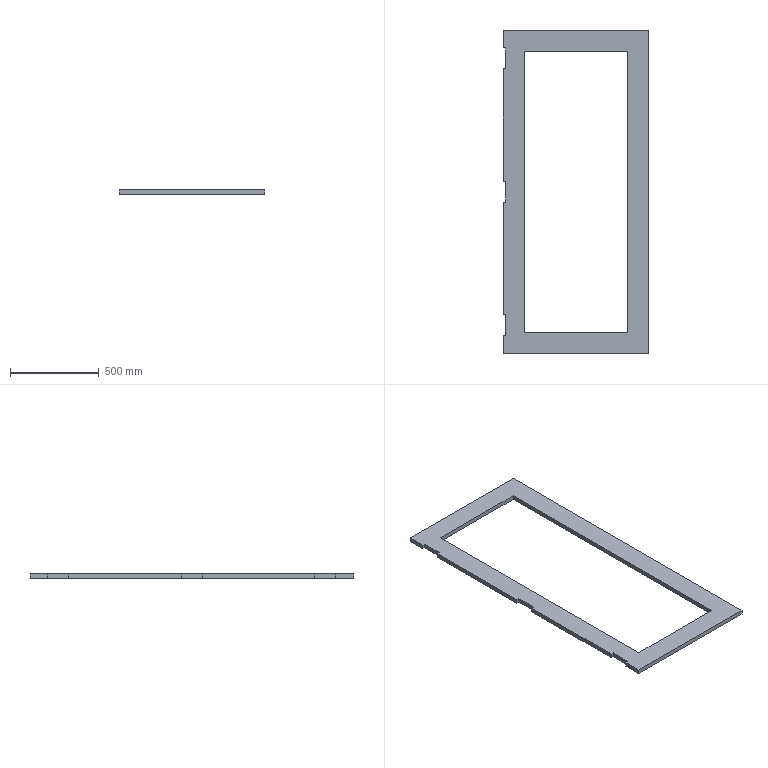Part | SolidWorks | features ICE 2, Extrusion 1 | 1 solid | 22 faces | box 820 x 1820 x 25 mm | volume 14268375 mm3 | plane 22
STEP:
#1=CARTESIAN_POINT('',(-410.,693.,0.));
#2=VERTEX_POINT('',#1);
#3=CARTESIAN_POINT('',(-410.,60.,0.));
#4=VERTEX_POINT('',#3);
#5=CARTESIAN_POINT('',(-410.,910.,0.));
#6=DIRECTION('',(0.,-1.,0.));
#7=VECTOR('',#6,1000.);
#8=LINE('',#5,#7);
#9=EDGE_CURVE('',#2,#4,#8,.T.);
#10=ORIENTED_EDGE('',*,*,#9,.T.);
#11=CARTESIAN_POINT('',(-410.,60.,25.));
#12=VERTEX_POINT('',#11);
#13=CARTESIAN_POINT('',(-410.,60.,0.));
#14=DIRECTION('',(0.,0.,1.));
#15=VECTOR('',#14,1000.);
#16=LINE('',#13,#15);
#17=EDGE_CURVE('',#4,#12,#16,.T.);
#18=ORIENTED_EDGE('',*,*,#17,.T.);
#19=CARTESIAN_POINT('',(-410.,693.,25.));
#20=VERTEX_POINT('',#19);
#21=CARTESIAN_POINT('',(-410.,910.,25.));
#22=DIRECTION('',(0.,-1.,0.));
#23=VECTOR('',#22,1000.);
#24=LINE('',#21,#23);
#25=EDGE_CURVE('',#20,#12,#24,.T.);
#26=ORIENTED_EDGE('',*,*,#25,.F.);
#27=CARTESIAN_POINT('',(-410.,693.,0.));
#28=DIRECTION('',(0.,0.,1.));
#29=VECTOR('',#28,1000.);
#30=LINE('',#27,#29);
#31=EDGE_CURVE('',#2,#20,#30,.T.);
#32=ORIENTED_EDGE('',*,*,#31,.F.);
#33=EDGE_LOOP('',(#10,#18,#26,#32));
#34=FACE_OUTER_BOUND('',#33,.T.);
#35=CARTESIAN_POINT('',(-410.,910.,25.));
#36=DIRECTION('',(1.,0.,0.));
#37=DIRECTION('',(0.,1.,0.));
#38=AXIS2_PLACEMENT_3D('',#35,#36,#37);
#39=PLANE('',#38);
#40=ADVANCED_FACE('',(#34),#39,.F.);
#41=CARTESIAN_POINT('',(-410.,910.,0.));
#42=VERTEX_POINT('',#41);
#43=CARTESIAN_POINT('',(-410.,810.,0.));
#44=VERTEX_POINT('',#43);
#45=CARTESIAN_POINT('',(-410.,910.,0.));
#46=DIRECTION('',(0.,-1.,0.));
#47=VECTOR('',#46,1000.);
#48=LINE('',#45,#47);
#49=EDGE_CURVE('',#42,#44,#48,.T.);
#50=ORIENTED_EDGE('',*,*,#49,.T.);
#51=CARTESIAN_POINT('',(-410.,810.,25.));
#52=VERTEX_POINT('',#51);
#53=CARTESIAN_POINT('',(-410.,810.,0.));
#54=DIRECTION('',(0.,0.,1.));
#55=VECTOR('',#54,1000.);
#56=LINE('',#53,#55);
#57=EDGE_CURVE('',#44,#52,#56,.T.);
#58=ORIENTED_EDGE('',*,*,#57,.T.);
#59=CARTESIAN_POINT('',(-410.,910.,25.));
#60=VERTEX_POINT('',#59);
#61=CARTESIAN_POINT('',(-410.,910.,25.));
#62=DIRECTION('',(0.,-1.,0.));
#63=VECTOR('',#62,1000.);
#64=LINE('',#61,#63);
#65=EDGE_CURVE('',#60,#52,#64,.T.);
#66=ORIENTED_EDGE('',*,*,#65,.F.);
#67=CARTESIAN_POINT('',(-410.,910.,25.));
#68=DIRECTION('',(0.,0.,-1.));
#69=VECTOR('',#68,1000.);
#70=LINE('',#67,#69);
#71=EDGE_CURVE('',#60,#42,#70,.T.);
#72=ORIENTED_EDGE('',*,*,#71,.T.);
#73=EDGE_LOOP('',(#50,#58,#66,#72));
#74=FACE_OUTER_BOUND('',#73,.T.);
#75=CARTESIAN_POINT('',(-410.,910.,25.));
#76=DIRECTION('',(1.,0.,0.));
#77=DIRECTION('',(0.,1.,0.));
#78=AXIS2_PLACEMENT_3D('',#75,#76,#77);
#79=PLANE('',#78);
#80=ADVANCED_FACE('',(#74),#79,.F.);
#81=CARTESIAN_POINT('',(-410.,-57.,25.));
#82=VERTEX_POINT('',#81);
#83=CARTESIAN_POINT('',(-410.,-690.,25.));
#84=VERTEX_POINT('',#83);
#85=CARTESIAN_POINT('',(-410.,910.,25.));
#86=DIRECTION('',(0.,-1.,0.));
#87=VECTOR('',#86,1000.);
#88=LINE('',#85,#87);
#89=EDGE_CURVE('',#82,#84,#88,.T.);
#90=ORIENTED_EDGE('',*,*,#89,.F.);
#91=CARTESIAN_POINT('',(-410.,-57.,0.));
#92=VERTEX_POINT('',#91);
#93=CARTESIAN_POINT('',(-410.,-57.,0.));
#94=DIRECTION('',(0.,0.,1.));
#95=VECTOR('',#94,1000.);
#96=LINE('',#93,#95);
#97=EDGE_CURVE('',#92,#82,#96,.T.);
#98=ORIENTED_EDGE('',*,*,#97,.F.);
#99=CARTESIAN_POINT('',(-410.,-690.,0.));
#100=VERTEX_POINT('',#99);
#101=CARTESIAN_POINT('',(-410.,910.,0.));
#102=DIRECTION('',(0.,-1.,0.));
#103=VECTOR('',#102,1000.);
#104=LINE('',#101,#103);
#105=EDGE_CURVE('',#92,#100,#104,.T.);
#106=ORIENTED_EDGE('',*,*,#105,.T.);
#107=CARTESIAN_POINT('',(-410.,-690.,0.));
#108=DIRECTION('',(0.,0.,1.));
#109=VECTOR('',#108,1000.);
#110=LINE('',#107,#109);
#111=EDGE_CURVE('',#100,#84,#110,.T.);
#112=ORIENTED_EDGE('',*,*,#111,.T.);
#113=EDGE_LOOP('',(#90,#98,#106,#112));
#114=FACE_OUTER_BOUND('',#113,.T.);
#115=CARTESIAN_POINT('',(-410.,910.,25.));
#116=DIRECTION('',(1.,0.,0.));
#117=DIRECTION('',(0.,1.,0.));
#118=AXIS2_PLACEMENT_3D('',#115,#116,#117);
#119=PLANE('',#118);
#120=ADVANCED_FACE('',(#114),#119,.F.);
#121=CARTESIAN_POINT('',(410.,-910.,0.));
#122=VERTEX_POINT('',#121);
#123=CARTESIAN_POINT('',(410.,910.,0.));
#124=VERTEX_POINT('',#123);
#125=CARTESIAN_POINT('',(410.,910.,0.));
#126=DIRECTION('',(0.,1.,0.));
#127=VECTOR('',#126,1000.);
#128=LINE('',#125,#127);
#129=EDGE_CURVE('',#122,#124,#128,.T.);
#130=ORIENTED_EDGE('',*,*,#129,.T.);
#131=CARTESIAN_POINT('',(410.,910.,25.));
#132=VERTEX_POINT('',#131);
#133=CARTESIAN_POINT('',(410.,910.,25.));
#134=DIRECTION('',(0.,0.,-1.));
#135=VECTOR('',#134,1000.);
#136=LINE('',#133,#135);
#137=EDGE_CURVE('',#132,#124,#136,.T.);
#138=ORIENTED_EDGE('',*,*,#137,.F.);
#139=CARTESIAN_POINT('',(410.,-910.,25.));
#140=VERTEX_POINT('',#139);
#141=CARTESIAN_POINT('',(410.,910.,25.));
#142=DIRECTION('',(0.,1.,0.));
#143=VECTOR('',#142,1000.);
#144=LINE('',#141,#143);
#145=EDGE_CURVE('',#140,#132,#144,.T.);
#146=ORIENTED_EDGE('',*,*,#145,.F.);
#147=CARTESIAN_POINT('',(410.,-910.,25.));
#148=DIRECTION('',(0.,0.,-1.));
#149=VECTOR('',#148,1000.);
#150=LINE('',#147,#149);
#151=EDGE_CURVE('',#140,#122,#150,.T.);
#152=ORIENTED_EDGE('',*,*,#151,.T.);
#153=EDGE_LOOP('',(#130,#138,#146,#152));
#154=FACE_OUTER_BOUND('',#153,.T.);
#155=CARTESIAN_POINT('',(410.,910.,25.));
#156=DIRECTION('',(-1.,0.,0.));
#157=DIRECTION('',(0.,-1.,0.));
#158=AXIS2_PLACEMENT_3D('',#155,#156,#157);
#159=PLANE('',#158);
#160=ADVANCED_FACE('',(#154),#159,.F.);
#161=CARTESIAN_POINT('',(-410.,910.,0.));
#162=DIRECTION('',(-1.,0.,0.));
#163=VECTOR('',#162,1000.);
#164=LINE('',#161,#163);
#165=EDGE_CURVE('',#124,#42,#164,.T.);
#166=ORIENTED_EDGE('',*,*,#165,.T.);
#167=ORIENTED_EDGE('',*,*,#71,.F.);
#168=CARTESIAN_POINT('',(-410.,910.,25.));
#169=DIRECTION('',(-1.,0.,0.));
#170=VECTOR('',#169,1000.);
#171=LINE('',#168,#170);
#172=EDGE_CURVE('',#132,#60,#171,.T.);
#173=ORIENTED_EDGE('',*,*,#172,.F.);
#174=ORIENTED_EDGE('',*,*,#137,.T.);
#175=EDGE_LOOP('',(#166,#167,#173,#174));
#176=FACE_OUTER_BOUND('',#175,.T.);
#177=CARTESIAN_POINT('',(-410.,910.,25.));
#178=DIRECTION('',(0.,-1.,0.));
#179=DIRECTION('',(0.,0.,-1.));
#180=AXIS2_PLACEMENT_3D('',#177,#178,#179);
#181=PLANE('',#180);
#182=ADVANCED_FACE('',(#176),#181,.F.);
#183=CARTESIAN_POINT('',(-410.,-807.,25.));
#184=VERTEX_POINT('',#183);
#185=CARTESIAN_POINT('',(-410.,-910.,25.));
#186=VERTEX_POINT('',#185);
#187=CARTESIAN_POINT('',(-410.,910.,25.));
#188=DIRECTION('',(0.,-1.,0.));
#189=VECTOR('',#188,1000.);
#190=LINE('',#187,#189);
#191=EDGE_CURVE('',#184,#186,#190,.T.);
#192=ORIENTED_EDGE('',*,*,#191,.F.);
#193=CARTESIAN_POINT('',(-410.,-807.,0.));
#194=VERTEX_POINT('',#193);
#195=CARTESIAN_POINT('',(-410.,-807.,0.));
#196=DIRECTION('',(0.,0.,1.));
#197=VECTOR('',#196,1000.);
#198=LINE('',#195,#197);
#199=EDGE_CURVE('',#194,#184,#198,.T.);
#200=ORIENTED_EDGE('',*,*,#199,.F.);
#201=CARTESIAN_POINT('',(-410.,-910.,0.));
#202=VERTEX_POINT('',#201);
#203=CARTESIAN_POINT('',(-410.,910.,0.));
#204=DIRECTION('',(0.,-1.,0.));
#205=VECTOR('',#204,1000.);
#206=LINE('',#203,#205);
#207=EDGE_CURVE('',#194,#202,#206,.T.);
#208=ORIENTED_EDGE('',*,*,#207,.T.);
#209=CARTESIAN_POINT('',(-410.,-910.,25.));
#210=DIRECTION('',(0.,0.,-1.));
#211=VECTOR('',#210,1000.);
#212=LINE('',#209,#211);
#213=EDGE_CURVE('',#186,#202,#212,.T.);
#214=ORIENTED_EDGE('',*,*,#213,.F.);
#215=EDGE_LOOP('',(#192,#200,#208,#214));
#216=FACE_OUTER_BOUND('',#215,.T.);
#217=CARTESIAN_POINT('',(-410.,910.,25.));
#218=DIRECTION('',(1.,0.,0.));
#219=DIRECTION('',(0.,1.,0.));
#220=AXIS2_PLACEMENT_3D('',#217,#218,#219);
#221=PLANE('',#220);
#222=ADVANCED_FACE('',(#216),#221,.F.);
#223=CARTESIAN_POINT('',(-410.,-910.,0.));
#224=DIRECTION('',(1.,0.,0.));
#225=VECTOR('',#224,1000.);
#226=LINE('',#223,#225);
#227=EDGE_CURVE('',#202,#122,#226,.T.);
#228=ORIENTED_EDGE('',*,*,#227,.T.);
#229=ORIENTED_EDGE('',*,*,#151,.F.);
#230=CARTESIAN_POINT('',(-410.,-910.,25.));
#231=DIRECTION('',(1.,0.,0.));
#232=VECTOR('',#231,1000.);
#233=LINE('',#230,#232);
#234=EDGE_CURVE('',#186,#140,#233,.T.);
#235=ORIENTED_EDGE('',*,*,#234,.F.);
#236=ORIENTED_EDGE('',*,*,#213,.T.);
#237=EDGE_LOOP('',(#228,#229,#235,#236));
#238=FACE_OUTER_BOUND('',#237,.T.);
#239=CARTESIAN_POINT('',(-410.,-910.,25.));
#240=DIRECTION('',(0.,1.,0.));
#241=DIRECTION('',(0.,0.,1.));
#242=AXIS2_PLACEMENT_3D('',#239,#240,#241);
#243=PLANE('',#242);
#244=ADVANCED_FACE('',(#238),#243,.F.);
#245=CARTESIAN_POINT('',(-395.,60.,25.));
#246=VERTEX_POINT('',#245);
#247=CARTESIAN_POINT('',(-410.,60.,25.));
#248=DIRECTION('',(-1.,0.,0.));
#249=VECTOR('',#248,1000.);
#250=LINE('',#247,#249);
#251=EDGE_CURVE('',#246,#12,#250,.T.);
#252=ORIENTED_EDGE('',*,*,#251,.F.);
#253=CARTESIAN_POINT('',(-395.,-57.,25.));
#254=VERTEX_POINT('',#253);
#255=CARTESIAN_POINT('',(-395.,60.,25.));
#256=DIRECTION('',(0.,1.,0.));
#257=VECTOR('',#256,1000.);
#258=LINE('',#255,#257);
#259=EDGE_CURVE('',#254,#246,#258,.T.);
#260=ORIENTED_EDGE('',*,*,#259,.F.);
#261=CARTESIAN_POINT('',(-410.,-57.,25.));
#262=DIRECTION('',(1.,0.,0.));
#263=VECTOR('',#262,1000.);
#264=LINE('',#261,#263);
#265=EDGE_CURVE('',#82,#254,#264,.T.);
#266=ORIENTED_EDGE('',*,*,#265,.F.);
#267=ORIENTED_EDGE('',*,*,#89,.T.);
#268=CARTESIAN_POINT('',(-395.,-690.,25.));
#269=VERTEX_POINT('',#268);
#270=CARTESIAN_POINT('',(-410.,-690.,25.));
#271=DIRECTION('',(-1.,0.,0.));
#272=VECTOR('',#271,1000.);
#273=LINE('',#270,#272);
#274=EDGE_CURVE('',#269,#84,#273,.T.);
#275=ORIENTED_EDGE('',*,*,#274,.F.);
#276=CARTESIAN_POINT('',(-395.,-807.,25.));
#277=VERTEX_POINT('',#276);
#278=CARTESIAN_POINT('',(-395.,-690.,25.));
#279=DIRECTION('',(0.,1.,0.));
#280=VECTOR('',#279,1000.);
#281=LINE('',#278,#280);
#282=EDGE_CURVE('',#277,#269,#281,.T.);
#283=ORIENTED_EDGE('',*,*,#282,.F.);
#284=CARTESIAN_POINT('',(-410.,-807.,25.));
#285=DIRECTION('',(1.,0.,0.));
#286=VECTOR('',#285,1000.);
#287=LINE('',#284,#286);
#288=EDGE_CURVE('',#184,#277,#287,.T.);
#289=ORIENTED_EDGE('',*,*,#288,.F.);
#290=ORIENTED_EDGE('',*,*,#191,.T.);
#291=ORIENTED_EDGE('',*,*,#234,.T.);
#292=ORIENTED_EDGE('',*,*,#145,.T.);
#293=ORIENTED_EDGE('',*,*,#172,.T.);
#294=ORIENTED_EDGE('',*,*,#65,.T.);
#295=CARTESIAN_POINT('',(-395.,810.,25.));
#296=VERTEX_POINT('',#295);
#297=CARTESIAN_POINT('',(-410.,810.,25.));
#298=DIRECTION('',(-1.,0.,0.));
#299=VECTOR('',#298,1000.);
#300=LINE('',#297,#299);
#301=EDGE_CURVE('',#296,#52,#300,.T.);
#302=ORIENTED_EDGE('',*,*,#301,.F.);
#303=CARTESIAN_POINT('',(-395.,693.,25.));
#304=VERTEX_POINT('',#303);
#305=CARTESIAN_POINT('',(-395.,810.,25.));
#306=DIRECTION('',(0.,1.,0.));
#307=VECTOR('',#306,1000.);
#308=LINE('',#305,#307);
#309=EDGE_CURVE('',#304,#296,#308,.T.);
#310=ORIENTED_EDGE('',*,*,#309,.F.);
#311=CARTESIAN_POINT('',(-410.,693.,25.));
#312=DIRECTION('',(1.,0.,0.));
#313=VECTOR('',#312,1000.);
#314=LINE('',#311,#313);
#315=EDGE_CURVE('',#20,#304,#314,.T.);
#316=ORIENTED_EDGE('',*,*,#315,.F.);
#317=ORIENTED_EDGE('',*,*,#25,.T.);
#318=EDGE_LOOP('',(#252,#260,#266,#267,#275,#283,#289,#290,#291,#292,#293,#294,#302,#310,#316,#317));
#319=FACE_OUTER_BOUND('',#318,.T.);
#320=CARTESIAN_POINT('',(290.,-790.,25.));
#321=VERTEX_POINT('',#320);
#322=CARTESIAN_POINT('',(290.,790.,25.));
#323=VERTEX_POINT('',#322);
#324=CARTESIAN_POINT('',(290.,-790.,25.));
#325=DIRECTION('',(0.,1.,0.));
#326=VECTOR('',#325,1000.);
#327=LINE('',#324,#326);
#328=EDGE_CURVE('',#321,#323,#327,.T.);
#329=ORIENTED_EDGE('',*,*,#328,.F.);
#330=CARTESIAN_POINT('',(-290.,-790.,25.));
#331=VERTEX_POINT('',#330);
#332=CARTESIAN_POINT('',(-290.,-790.,25.));
#333=DIRECTION('',(1.,0.,0.));
#334=VECTOR('',#333,1000.);
#335=LINE('',#332,#334);
#336=EDGE_CURVE('',#331,#321,#335,.T.);
#337=ORIENTED_EDGE('',*,*,#336,.F.);
#338=CARTESIAN_POINT('',(-290.,790.,25.));
#339=VERTEX_POINT('',#338);
#340=CARTESIAN_POINT('',(-290.,-790.,25.));
#341=DIRECTION('',(0.,-1.,0.));
#342=VECTOR('',#341,1000.);
#343=LINE('',#340,#342);
#344=EDGE_CURVE('',#339,#331,#343,.T.);
#345=ORIENTED_EDGE('',*,*,#344,.F.);
#346=CARTESIAN_POINT('',(-290.,790.,25.));
#347=DIRECTION('',(-1.,0.,0.));
#348=VECTOR('',#347,1000.);
#349=LINE('',#346,#348);
#350=EDGE_CURVE('',#323,#339,#349,.T.);
#351=ORIENTED_EDGE('',*,*,#350,.F.);
#352=EDGE_LOOP('',(#329,#337,#345,#351));
#353=FACE_BOUND('',#352,.T.);
#354=CARTESIAN_POINT('',(0.,0.,25.));
#355=DIRECTION('',(0.,0.,1.));
#356=DIRECTION('',(1.,0.,0.));
#357=AXIS2_PLACEMENT_3D('',#354,#355,#356);
#358=PLANE('',#357);
#359=ADVANCED_FACE('',(#319,#353),#358,.T.);
#360=CARTESIAN_POINT('',(-290.,-790.,0.));
#361=VERTEX_POINT('',#360);
#362=CARTESIAN_POINT('',(290.,-790.,0.));
#363=VERTEX_POINT('',#362);
#364=CARTESIAN_POINT('',(-290.,-790.,0.));
#365=DIRECTION('',(1.,0.,0.));
#366=VECTOR('',#365,1000.);
#367=LINE('',#364,#366);
#368=EDGE_CURVE('',#361,#363,#367,.T.);
#369=ORIENTED_EDGE('',*,*,#368,.T.);
#370=CARTESIAN_POINT('',(290.,790.,0.));
#371=VERTEX_POINT('',#370);
#372=CARTESIAN_POINT('',(290.,-790.,0.));
#373=DIRECTION('',(0.,1.,0.));
#374=VECTOR('',#373,1000.);
#375=LINE('',#372,#374);
#376=EDGE_CURVE('',#363,#371,#375,.T.);
#377=ORIENTED_EDGE('',*,*,#376,.T.);
#378=CARTESIAN_POINT('',(-290.,790.,0.));
#379=VERTEX_POINT('',#378);
#380=CARTESIAN_POINT('',(-290.,790.,0.));
#381=DIRECTION('',(-1.,0.,0.));
#382=VECTOR('',#381,1000.);
#383=LINE('',#380,#382);
#384=EDGE_CURVE('',#371,#379,#383,.T.);
#385=ORIENTED_EDGE('',*,*,#384,.T.);
#386=CARTESIAN_POINT('',(-290.,-790.,0.));
#387=DIRECTION('',(0.,-1.,0.));
#388=VECTOR('',#387,1000.);
#389=LINE('',#386,#388);
#390=EDGE_CURVE('',#379,#361,#389,.T.);
#391=ORIENTED_EDGE('',*,*,#390,.T.);
#392=EDGE_LOOP('',(#369,#377,#385,#391));
#393=FACE_BOUND('',#392,.T.);
#394=CARTESIAN_POINT('',(-395.,-57.,0.));
#395=VERTEX_POINT('',#394);
#396=CARTESIAN_POINT('',(-395.,60.,0.));
#397=VERTEX_POINT('',#396);
#398=CARTESIAN_POINT('',(-395.,60.,0.));
#399=DIRECTION('',(0.,1.,0.));
#400=VECTOR('',#399,1000.);
#401=LINE('',#398,#400);
#402=EDGE_CURVE('',#395,#397,#401,.T.);
#403=ORIENTED_EDGE('',*,*,#402,.T.);
#404=CARTESIAN_POINT('',(-410.,60.,0.));
#405=DIRECTION('',(-1.,0.,0.));
#406=VECTOR('',#405,1000.);
#407=LINE('',#404,#406);
#408=EDGE_CURVE('',#397,#4,#407,.T.);
#409=ORIENTED_EDGE('',*,*,#408,.T.);
#410=ORIENTED_EDGE('',*,*,#9,.F.);
#411=CARTESIAN_POINT('',(-395.,693.,0.));
#412=VERTEX_POINT('',#411);
#413=CARTESIAN_POINT('',(-410.,693.,0.));
#414=DIRECTION('',(1.,0.,0.));
#415=VECTOR('',#414,1000.);
#416=LINE('',#413,#415);
#417=EDGE_CURVE('',#2,#412,#416,.T.);
#418=ORIENTED_EDGE('',*,*,#417,.T.);
#419=CARTESIAN_POINT('',(-395.,810.,0.));
#420=VERTEX_POINT('',#419);
#421=CARTESIAN_POINT('',(-395.,810.,0.));
#422=DIRECTION('',(0.,1.,0.));
#423=VECTOR('',#422,1000.);
#424=LINE('',#421,#423);
#425=EDGE_CURVE('',#412,#420,#424,.T.);
#426=ORIENTED_EDGE('',*,*,#425,.T.);
#427=CARTESIAN_POINT('',(-410.,810.,0.));
#428=DIRECTION('',(-1.,0.,0.));
#429=VECTOR('',#428,1000.);
#430=LINE('',#427,#429);
#431=EDGE_CURVE('',#420,#44,#430,.T.);
#432=ORIENTED_EDGE('',*,*,#431,.T.);
#433=ORIENTED_EDGE('',*,*,#49,.F.);
#434=ORIENTED_EDGE('',*,*,#165,.F.);
#435=ORIENTED_EDGE('',*,*,#129,.F.);
#436=ORIENTED_EDGE('',*,*,#227,.F.);
#437=ORIENTED_EDGE('',*,*,#207,.F.);
#438=CARTESIAN_POINT('',(-395.,-807.,0.));
#439=VERTEX_POINT('',#438);
#440=CARTESIAN_POINT('',(-410.,-807.,0.));
#441=DIRECTION('',(1.,0.,0.));
#442=VECTOR('',#441,1000.);
#443=LINE('',#440,#442);
#444=EDGE_CURVE('',#194,#439,#443,.T.);
#445=ORIENTED_EDGE('',*,*,#444,.T.);
#446=CARTESIAN_POINT('',(-395.,-690.,0.));
#447=VERTEX_POINT('',#446);
#448=CARTESIAN_POINT('',(-395.,-690.,0.));
#449=DIRECTION('',(0.,1.,0.));
#450=VECTOR('',#449,1000.);
#451=LINE('',#448,#450);
#452=EDGE_CURVE('',#439,#447,#451,.T.);
#453=ORIENTED_EDGE('',*,*,#452,.T.);
#454=CARTESIAN_POINT('',(-410.,-690.,0.));
#455=DIRECTION('',(-1.,0.,0.));
#456=VECTOR('',#455,1000.);
#457=LINE('',#454,#456);
#458=EDGE_CURVE('',#447,#100,#457,.T.);
#459=ORIENTED_EDGE('',*,*,#458,.T.);
#460=ORIENTED_EDGE('',*,*,#105,.F.);
#461=CARTESIAN_POINT('',(-410.,-57.,0.));
#462=DIRECTION('',(1.,0.,0.));
#463=VECTOR('',#462,1000.);
#464=LINE('',#461,#463);
#465=EDGE_CURVE('',#92,#395,#464,.T.);
#466=ORIENTED_EDGE('',*,*,#465,.T.);
#467=EDGE_LOOP('',(#403,#409,#410,#418,#426,#432,#433,#434,#435,#436,#437,#445,#453,#459,#460,#466));
#468=FACE_OUTER_BOUND('',#467,.T.);
#469=CARTESIAN_POINT('',(0.,0.,0.));
#470=DIRECTION('',(0.,0.,1.));
#471=DIRECTION('',(1.,0.,0.));
#472=AXIS2_PLACEMENT_3D('',#469,#470,#471);
#473=PLANE('',#472);
#474=ADVANCED_FACE('',(#393,#468),#473,.F.);
#475=ORIENTED_EDGE('',*,*,#328,.T.);
#476=CARTESIAN_POINT('',(290.,790.,0.));
#477=DIRECTION('',(0.,0.,1.));
#478=VECTOR('',#477,1000.);
#479=LINE('',#476,#478);
#480=EDGE_CURVE('',#371,#323,#479,.T.);
#481=ORIENTED_EDGE('',*,*,#480,.F.);
#482=ORIENTED_EDGE('',*,*,#376,.F.);
#483=CARTESIAN_POINT('',(290.,-790.,0.));
#484=DIRECTION('',(0.,0.,1.));
#485=VECTOR('',#484,1000.);
#486=LINE('',#483,#485);
#487=EDGE_CURVE('',#363,#321,#486,.T.);
#488=ORIENTED_EDGE('',*,*,#487,.T.);
#489=EDGE_LOOP('',(#475,#481,#482,#488));
#490=FACE_OUTER_BOUND('',#489,.T.);
#491=CARTESIAN_POINT('',(290.,-790.,0.));
#492=DIRECTION('',(1.,0.,0.));
#493=DIRECTION('',(0.,0.,-1.));
#494=AXIS2_PLACEMENT_3D('',#491,#492,#493);
#495=PLANE('',#494);
#496=ADVANCED_FACE('',(#490),#495,.F.);
#497=ORIENTED_EDGE('',*,*,#336,.T.);
#498=ORIENTED_EDGE('',*,*,#487,.F.);
#499=ORIENTED_EDGE('',*,*,#368,.F.);
#500=CARTESIAN_POINT('',(-290.,-790.,0.));
#501=DIRECTION('',(0.,0.,1.));
#502=VECTOR('',#501,1000.);
#503=LINE('',#500,#502);
#504=EDGE_CURVE('',#361,#331,#503,.T.);
#505=ORIENTED_EDGE('',*,*,#504,.T.);
#506=EDGE_LOOP('',(#497,#498,#499,#505));
#507=FACE_OUTER_BOUND('',#506,.T.);
#508=CARTESIAN_POINT('',(-290.,-790.,0.));
#509=DIRECTION('',(0.,-1.,0.));
#510=DIRECTION('',(0.,0.,-1.));
#511=AXIS2_PLACEMENT_3D('',#508,#509,#510);
#512=PLANE('',#511);
#513=ADVANCED_FACE('',(#507),#512,.F.);
#514=ORIENTED_EDGE('',*,*,#344,.T.);
#515=ORIENTED_EDGE('',*,*,#504,.F.);
#516=ORIENTED_EDGE('',*,*,#390,.F.);
#517=CARTESIAN_POINT('',(-290.,790.,0.));
#518=DIRECTION('',(0.,0.,1.));
#519=VECTOR('',#518,1000.);
#520=LINE('',#517,#519);
#521=EDGE_CURVE('',#379,#339,#520,.T.);
#522=ORIENTED_EDGE('',*,*,#521,.T.);
#523=EDGE_LOOP('',(#514,#515,#516,#522));
#524=FACE_OUTER_BOUND('',#523,.T.);
#525=CARTESIAN_POINT('',(-290.,-790.,0.));
#526=DIRECTION('',(-1.,0.,0.));
#527=DIRECTION('',(0.,0.,1.));
#528=AXIS2_PLACEMENT_3D('',#525,#526,#527);
#529=PLANE('',#528);
#530=ADVANCED_FACE('',(#524),#529,.F.);
#531=ORIENTED_EDGE('',*,*,#350,.T.);
#532=ORIENTED_EDGE('',*,*,#521,.F.);
#533=ORIENTED_EDGE('',*,*,#384,.F.);
#534=ORIENTED_EDGE('',*,*,#480,.T.);
#535=EDGE_LOOP('',(#531,#532,#533,#534));
#536=FACE_OUTER_BOUND('',#535,.T.);
#537=CARTESIAN_POINT('',(-290.,790.,0.));
#538=DIRECTION('',(0.,1.,0.));
#539=DIRECTION('',(0.,0.,1.));
#540=AXIS2_PLACEMENT_3D('',#537,#538,#539);
#541=PLANE('',#540);
#542=ADVANCED_FACE('',(#536),#541,.F.);
#543=ORIENTED_EDGE('',*,*,#274,.T.);
#544=ORIENTED_EDGE('',*,*,#111,.F.);
#545=ORIENTED_EDGE('',*,*,#458,.F.);
#546=CARTESIAN_POINT('',(-395.,-690.,0.));
#547=DIRECTION('',(0.,0.,1.));
#548=VECTOR('',#547,1000.);
#549=LINE('',#546,#548);
#550=EDGE_CURVE('',#447,#269,#549,.T.);
#551=ORIENTED_EDGE('',*,*,#550,.T.);
#552=EDGE_LOOP('',(#543,#544,#545,#551));
#553=FACE_OUTER_BOUND('',#552,.T.);
#554=CARTESIAN_POINT('',(-410.,-690.,0.));
#555=DIRECTION('',(0.,1.,0.));
#556=DIRECTION('',(0.,0.,1.));
#557=AXIS2_PLACEMENT_3D('',#554,#555,#556);
#558=PLANE('',#557);
#559=ADVANCED_FACE('',(#553),#558,.F.);
#560=ORIENTED_EDGE('',*,*,#282,.T.);
#561=ORIENTED_EDGE('',*,*,#550,.F.);
#562=ORIENTED_EDGE('',*,*,#452,.F.);
#563=CARTESIAN_POINT('',(-395.,-807.,0.));
#564=DIRECTION('',(0.,0.,1.));
#565=VECTOR('',#564,1000.);
#566=LINE('',#563,#565);
#567=EDGE_CURVE('',#439,#277,#566,.T.);
#568=ORIENTED_EDGE('',*,*,#567,.T.);
#569=EDGE_LOOP('',(#560,#561,#562,#568));
#570=FACE_OUTER_BOUND('',#569,.T.);
#571=CARTESIAN_POINT('',(-395.,-690.,0.));
#572=DIRECTION('',(1.,0.,0.));
#573=DIRECTION('',(0.,0.,-1.));
#574=AXIS2_PLACEMENT_3D('',#571,#572,#573);
#575=PLANE('',#574);
#576=ADVANCED_FACE('',(#570),#575,.F.);
#577=ORIENTED_EDGE('',*,*,#288,.T.);
#578=ORIENTED_EDGE('',*,*,#567,.F.);
#579=ORIENTED_EDGE('',*,*,#444,.F.);
#580=ORIENTED_EDGE('',*,*,#199,.T.);
#581=EDGE_LOOP('',(#577,#578,#579,#580));
#582=FACE_OUTER_BOUND('',#581,.T.);
#583=CARTESIAN_POINT('',(-410.,-807.,0.));
#584=DIRECTION('',(0.,-1.,0.));
#585=DIRECTION('',(0.,0.,-1.));
#586=AXIS2_PLACEMENT_3D('',#583,#584,#585);
#587=PLANE('',#586);
#588=ADVANCED_FACE('',(#582),#587,.F.);
#589=ORIENTED_EDGE('',*,*,#301,.T.);
#590=ORIENTED_EDGE('',*,*,#57,.F.);
#591=ORIENTED_EDGE('',*,*,#431,.F.);
#592=CARTESIAN_POINT('',(-395.,810.,0.));
#593=DIRECTION('',(0.,0.,1.));
#594=VECTOR('',#593,1000.);
#595=LINE('',#592,#594);
#596=EDGE_CURVE('',#420,#296,#595,.T.);
#597=ORIENTED_EDGE('',*,*,#596,.T.);
#598=EDGE_LOOP('',(#589,#590,#591,#597));
#599=FACE_OUTER_BOUND('',#598,.T.);
#600=CARTESIAN_POINT('',(-410.,810.,0.));
#601=DIRECTION('',(0.,1.,0.));
#602=DIRECTION('',(0.,0.,1.));
#603=AXIS2_PLACEMENT_3D('',#600,#601,#602);
#604=PLANE('',#603);
#605=ADVANCED_FACE('',(#599),#604,.F.);
#606=ORIENTED_EDGE('',*,*,#309,.T.);
#607=ORIENTED_EDGE('',*,*,#596,.F.);
#608=ORIENTED_EDGE('',*,*,#425,.F.);
#609=CARTESIAN_POINT('',(-395.,693.,0.));
#610=DIRECTION('',(0.,0.,1.));
#611=VECTOR('',#610,1000.);
#612=LINE('',#609,#611);
#613=EDGE_CURVE('',#412,#304,#612,.T.);
#614=ORIENTED_EDGE('',*,*,#613,.T.);
#615=EDGE_LOOP('',(#606,#607,#608,#614));
#616=FACE_OUTER_BOUND('',#615,.T.);
#617=CARTESIAN_POINT('',(-395.,810.,0.));
#618=DIRECTION('',(1.,0.,0.));
#619=DIRECTION('',(0.,0.,-1.));
#620=AXIS2_PLACEMENT_3D('',#617,#618,#619);
#621=PLANE('',#620);
#622=ADVANCED_FACE('',(#616),#621,.F.);
#623=ORIENTED_EDGE('',*,*,#315,.T.);
#624=ORIENTED_EDGE('',*,*,#613,.F.);
#625=ORIENTED_EDGE('',*,*,#417,.F.);
#626=ORIENTED_EDGE('',*,*,#31,.T.);
#627=EDGE_LOOP('',(#623,#624,#625,#626));
#628=FACE_OUTER_BOUND('',#627,.T.);
#629=CARTESIAN_POINT('',(-410.,693.,0.));
#630=DIRECTION('',(0.,-1.,0.));
#631=DIRECTION('',(0.,0.,-1.));
#632=AXIS2_PLACEMENT_3D('',#629,#630,#631);
#633=PLANE('',#632);
#634=ADVANCED_FACE('',(#628),#633,.F.);
#635=ORIENTED_EDGE('',*,*,#251,.T.);
#636=ORIENTED_EDGE('',*,*,#17,.F.);
#637=ORIENTED_EDGE('',*,*,#408,.F.);
#638=CARTESIAN_POINT('',(-395.,60.,0.));
#639=DIRECTION('',(0.,0.,1.));
#640=VECTOR('',#639,1000.);
#641=LINE('',#638,#640);
#642=EDGE_CURVE('',#397,#246,#641,.T.);
#643=ORIENTED_EDGE('',*,*,#642,.T.);
#644=EDGE_LOOP('',(#635,#636,#637,#643));
#645=FACE_OUTER_BOUND('',#644,.T.);
#646=CARTESIAN_POINT('',(-410.,60.,0.));
#647=DIRECTION('',(0.,1.,0.));
#648=DIRECTION('',(0.,0.,1.));
#649=AXIS2_PLACEMENT_3D('',#646,#647,#648);
#650=PLANE('',#649);
#651=ADVANCED_FACE('',(#645),#650,.F.);
#652=ORIENTED_EDGE('',*,*,#259,.T.);
#653=ORIENTED_EDGE('',*,*,#642,.F.);
#654=ORIENTED_EDGE('',*,*,#402,.F.);
#655=CARTESIAN_POINT('',(-395.,-57.,0.));
#656=DIRECTION('',(0.,0.,1.));
#657=VECTOR('',#656,1000.);
#658=LINE('',#655,#657);
#659=EDGE_CURVE('',#395,#254,#658,.T.);
#660=ORIENTED_EDGE('',*,*,#659,.T.);
#661=EDGE_LOOP('',(#652,#653,#654,#660));
#662=FACE_OUTER_BOUND('',#661,.T.);
#663=CARTESIAN_POINT('',(-395.,60.,0.));
#664=DIRECTION('',(1.,0.,0.));
#665=DIRECTION('',(0.,0.,-1.));
#666=AXIS2_PLACEMENT_3D('',#663,#664,#665);
#667=PLANE('',#666);
#668=ADVANCED_FACE('',(#662),#667,.F.);
#669=ORIENTED_EDGE('',*,*,#265,.T.);
#670=ORIENTED_EDGE('',*,*,#659,.F.);
#671=ORIENTED_EDGE('',*,*,#465,.F.);
#672=ORIENTED_EDGE('',*,*,#97,.T.);
#673=EDGE_LOOP('',(#669,#670,#671,#672));
#674=FACE_OUTER_BOUND('',#673,.T.);
#675=CARTESIAN_POINT('',(-410.,-57.,0.));
#676=DIRECTION('',(0.,-1.,0.));
#677=DIRECTION('',(0.,0.,-1.));
#678=AXIS2_PLACEMENT_3D('',#675,#676,#677);
#679=PLANE('',#678);
#680=ADVANCED_FACE('',(#674),#679,.F.);
#681=CLOSED_SHELL('',(#40,#80,#120,#160,#182,#222,#244,#359,#474,#496,#513,#530,#542,#559,#576,#588,#605,#622,#634,#651,#668,#680));
#682=MANIFOLD_SOLID_BREP('',#681);
#683=CARTESIAN_POINT('',(0.,0.,0.));
#684=DIRECTION('',(0.,0.,1.));
#685=DIRECTION('',(1.,0.,0.));
#686=AXIS2_PLACEMENT_3D('',#683,#684,#685);
#687=(LENGTH_UNIT()NAMED_UNIT(*)SI_UNIT(.MILLI.,.METRE.));
#688=UNCERTAINTY_MEASURE_WITH_UNIT(LENGTH_MEASURE(0.00001),#687,'','');
#689=(NAMED_UNIT(*)PLANE_ANGLE_UNIT()SI_UNIT($,.RADIAN.));
#690=(NAMED_UNIT(*)SI_UNIT($,.STERADIAN.)SOLID_ANGLE_UNIT());
#691=(GEOMETRIC_REPRESENTATION_CONTEXT(3)GLOBAL_UNCERTAINTY_ASSIGNED_CONTEXT((#688))GLOBAL_UNIT_ASSIGNED_CONTEXT((#687,#689,#690))REPRESENTATION_CONTEXT('',''));
#692=ADVANCED_BREP_SHAPE_REPRESENTATION('',(#682,#686),#691);